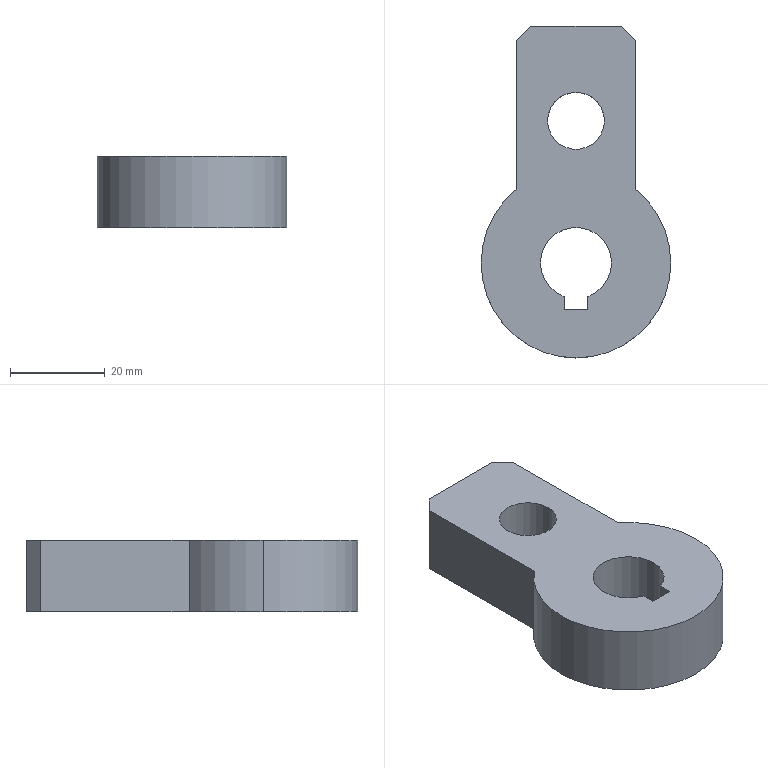Part | STEP file | 1 solid | 18 faces | box 40 x 70 x 15 mm | volume 25956 mm3 | plane 10 | cylinder 8 | commonest cylinder face diameters 15 x3 40 x3 12 x2
STEP:
#1=CARTESIAN_POINT('',(0.,0.,0.));
#2=DIRECTION('',(0.,0.,1.));
#3=DIRECTION('',(1.,0.,0.));
#4=AXIS2_PLACEMENT_3D('',#1,#2,#3);
#5=CARTESIAN_POINT('',(-6.,30.,7.5));
#6=VERTEX_POINT('',#5);
#7=CARTESIAN_POINT('',(-6.,30.,-7.5));
#8=VERTEX_POINT('',#7);
#9=CARTESIAN_POINT('',(-6.,30.,-7.5));
#10=DIRECTION('',(0.,0.,-1.));
#11=VECTOR('',#10,1.);
#12=LINE('',#9,#11);
#13=CARTESIAN_POINT('',(0.,30.,-7.5));
#14=DIRECTION('',(0.,0.,-1.));
#15=DIRECTION('',(-1.,0.,0.));
#16=AXIS2_PLACEMENT_3D('',#13,#14,#15);
#17=CYLINDRICAL_SURFACE('',#16,6.);
#18=CARTESIAN_POINT('',(6.283,0.));
#19=DIRECTION('',(0.,1.));
#20=VECTOR('',#19,1.);
#21=LINE('',#18,#20);
#22=(GEOMETRIC_REPRESENTATION_CONTEXT(2)PARAMETRIC_REPRESENTATION_CONTEXT()REPRESENTATION_CONTEXT('',''));
#23=DEFINITIONAL_REPRESENTATION('',(#21),#22);
#24=PCURVE('',#17,#23);
#25=CARTESIAN_POINT('',(0.,30.,-7.5));
#26=DIRECTION('',(0.,0.,-1.));
#27=DIRECTION('',(-1.,0.,0.));
#28=AXIS2_PLACEMENT_3D('',#25,#26,#27);
#29=CYLINDRICAL_SURFACE('',#28,6.);
#30=CARTESIAN_POINT('',(0.,0.));
#31=DIRECTION('',(0.,1.));
#32=VECTOR('',#31,1.);
#33=LINE('',#30,#32);
#34=(GEOMETRIC_REPRESENTATION_CONTEXT(2)PARAMETRIC_REPRESENTATION_CONTEXT()REPRESENTATION_CONTEXT('',''));
#35=DEFINITIONAL_REPRESENTATION('',(#33),#34);
#36=PCURVE('',#29,#35);
#37=SURFACE_CURVE('',#12,(#24,#36),.PCURVE_S1.);
#38=EDGE_CURVE('',#6,#8,#37,.T.);
#39=ORIENTED_EDGE('',*,*,#38,.T.);
#40=CARTESIAN_POINT('',(6.,30.,-7.5));
#41=VERTEX_POINT('',#40);
#42=CARTESIAN_POINT('',(0.,30.,-7.5));
#43=DIRECTION('',(0.,0.,1.));
#44=DIRECTION('',(-1.,0.,0.));
#45=AXIS2_PLACEMENT_3D('',#42,#43,#44);
#46=CIRCLE('',#45,6.);
#47=CARTESIAN_POINT('',(6.283,0.));
#48=DIRECTION('',(-1.,0.));
#49=VECTOR('',#48,1.);
#50=LINE('',#47,#49);
#51=(GEOMETRIC_REPRESENTATION_CONTEXT(2)PARAMETRIC_REPRESENTATION_CONTEXT()REPRESENTATION_CONTEXT('',''));
#52=DEFINITIONAL_REPRESENTATION('',(#50),#51);
#53=PCURVE('',#17,#52);
#54=CARTESIAN_POINT('',(0.,0.,-7.5));
#55=DIRECTION('',(0.,0.,1.));
#56=DIRECTION('',(1.,0.,0.));
#57=AXIS2_PLACEMENT_3D('',#54,#55,#56);
#58=PLANE('',#57);
#59=CARTESIAN_POINT('',(0.,30.));
#60=DIRECTION('',(-1.,0.));
#61=AXIS2_PLACEMENT_2D('',#59,#60);
#62=CIRCLE('',#61,6.);
#63=(GEOMETRIC_REPRESENTATION_CONTEXT(2)PARAMETRIC_REPRESENTATION_CONTEXT()REPRESENTATION_CONTEXT('',''));
#64=DEFINITIONAL_REPRESENTATION('',(#62),#63);
#65=PCURVE('',#58,#64);
#66=SURFACE_CURVE('',#46,(#53,#65),.PCURVE_S1.);
#67=EDGE_CURVE('',#8,#41,#66,.T.);
#68=ORIENTED_EDGE('',*,*,#67,.T.);
#69=CARTESIAN_POINT('',(6.,30.,7.5));
#70=VERTEX_POINT('',#69);
#71=CARTESIAN_POINT('',(6.,30.,-7.5));
#72=DIRECTION('',(0.,0.,-1.));
#73=VECTOR('',#72,1.);
#74=LINE('',#71,#73);
#75=CARTESIAN_POINT('',(3.142,0.));
#76=DIRECTION('',(0.,1.));
#77=VECTOR('',#76,1.);
#78=LINE('',#75,#77);
#79=(GEOMETRIC_REPRESENTATION_CONTEXT(2)PARAMETRIC_REPRESENTATION_CONTEXT()REPRESENTATION_CONTEXT('',''));
#80=DEFINITIONAL_REPRESENTATION('',(#78),#79);
#81=PCURVE('',#17,#80);
#82=CARTESIAN_POINT('',(3.142,0.));
#83=DIRECTION('',(0.,1.));
#84=VECTOR('',#83,1.);
#85=LINE('',#82,#84);
#86=(GEOMETRIC_REPRESENTATION_CONTEXT(2)PARAMETRIC_REPRESENTATION_CONTEXT()REPRESENTATION_CONTEXT('',''));
#87=DEFINITIONAL_REPRESENTATION('',(#85),#86);
#88=PCURVE('',#29,#87);
#89=SURFACE_CURVE('',#74,(#81,#88),.PCURVE_S1.);
#90=EDGE_CURVE('',#70,#41,#89,.T.);
#91=ORIENTED_EDGE('',*,*,#90,.F.);
#92=CARTESIAN_POINT('',(0.,30.,7.5));
#93=DIRECTION('',(0.,0.,-1.));
#94=DIRECTION('',(-1.,0.,0.));
#95=AXIS2_PLACEMENT_3D('',#92,#93,#94);
#96=CIRCLE('',#95,6.);
#97=CARTESIAN_POINT('',(0.,-15.));
#98=DIRECTION('',(1.,0.));
#99=VECTOR('',#98,1.);
#100=LINE('',#97,#99);
#101=(GEOMETRIC_REPRESENTATION_CONTEXT(2)PARAMETRIC_REPRESENTATION_CONTEXT()REPRESENTATION_CONTEXT('',''));
#102=DEFINITIONAL_REPRESENTATION('',(#100),#101);
#103=PCURVE('',#17,#102);
#104=CARTESIAN_POINT('',(0.,0.,7.5));
#105=DIRECTION('',(0.,0.,1.));
#106=DIRECTION('',(1.,0.,0.));
#107=AXIS2_PLACEMENT_3D('',#104,#105,#106);
#108=PLANE('',#107);
#109=CARTESIAN_POINT('',(-6.,30.));
#110=CARTESIAN_POINT('',(-6.,40.392));
#111=CARTESIAN_POINT('',(3.,35.196));
#112=CARTESIAN_POINT('',(12.,30.));
#113=CARTESIAN_POINT('',(3.,24.804));
#114=CARTESIAN_POINT('',(-6.,19.608));
#115=CARTESIAN_POINT('',(-6.,30.));
#116=(BOUNDED_CURVE()B_SPLINE_CURVE(2,(#109,#110,#111,#112,#113,#114,#115),.UNSPECIFIED.,.T.,.F.)B_SPLINE_CURVE_WITH_KNOTS((1,2,2,2,2,1),(-2.094,0.,2.094,4.189,6.283,8.378),.UNSPECIFIED.)CURVE()GEOMETRIC_REPRESENTATION_ITEM()RATIONAL_B_SPLINE_CURVE((1.,0.5,1.,0.5,1.,0.5,1.))REPRESENTATION_ITEM(''));
#117=(GEOMETRIC_REPRESENTATION_CONTEXT(2)PARAMETRIC_REPRESENTATION_CONTEXT()REPRESENTATION_CONTEXT('',''));
#118=DEFINITIONAL_REPRESENTATION('',(#116),#117);
#119=PCURVE('',#108,#118);
#120=SURFACE_CURVE('',#96,(#103,#119),.PCURVE_S1.);
#121=EDGE_CURVE('',#70,#6,#120,.T.);
#122=ORIENTED_EDGE('',*,*,#121,.T.);
#123=EDGE_LOOP('',(#39,#68,#91,#122));
#124=FACE_BOUND('',#123,.F.);
#125=ADVANCED_FACE('',(#124),#17,.F.);
#126=CARTESIAN_POINT('',(-2.5,-7.071,-7.5));
#127=VERTEX_POINT('',#126);
#128=CARTESIAN_POINT('',(-2.5,-7.071,7.5));
#129=VERTEX_POINT('',#128);
#130=CARTESIAN_POINT('',(-2.5,-7.071,7.5));
#131=DIRECTION('',(0.,0.,1.));
#132=VECTOR('',#131,1.);
#133=LINE('',#130,#132);
#134=CARTESIAN_POINT('',(0.,0.,7.5));
#135=DIRECTION('',(0.,0.,1.));
#136=DIRECTION('',(1.,0.,0.));
#137=AXIS2_PLACEMENT_3D('',#134,#135,#136);
#138=CYLINDRICAL_SURFACE('',#137,7.5);
#139=CARTESIAN_POINT('',(4.373,0.));
#140=DIRECTION('',(0.,1.));
#141=VECTOR('',#140,1.);
#142=LINE('',#139,#141);
#143=(GEOMETRIC_REPRESENTATION_CONTEXT(2)PARAMETRIC_REPRESENTATION_CONTEXT()REPRESENTATION_CONTEXT('',''));
#144=DEFINITIONAL_REPRESENTATION('',(#142),#143);
#145=PCURVE('',#138,#144);
#146=CARTESIAN_POINT('',(-2.5,-9.8,-7.5));
#147=DIRECTION('',(-1.,0.,0.));
#148=DIRECTION('',(0.,0.,1.));
#149=AXIS2_PLACEMENT_3D('',#146,#147,#148);
#150=PLANE('',#149);
#151=CARTESIAN_POINT('',(15.,2.729));
#152=DIRECTION('',(1.,0.));
#153=VECTOR('',#152,1.);
#154=LINE('',#151,#153);
#155=(GEOMETRIC_REPRESENTATION_CONTEXT(2)PARAMETRIC_REPRESENTATION_CONTEXT()REPRESENTATION_CONTEXT('',''));
#156=DEFINITIONAL_REPRESENTATION('',(#154),#155);
#157=PCURVE('',#150,#156);
#158=SURFACE_CURVE('',#133,(#145,#157),.PCURVE_S1.);
#159=EDGE_CURVE('',#127,#129,#158,.T.);
#160=ORIENTED_EDGE('',*,*,#159,.T.);
#161=CARTESIAN_POINT('',(-7.5,0.,7.5));
#162=VERTEX_POINT('',#161);
#163=CARTESIAN_POINT('',(0.,0.,7.5));
#164=DIRECTION('',(0.,0.,-1.));
#165=DIRECTION('',(1.,0.,0.));
#166=AXIS2_PLACEMENT_3D('',#163,#164,#165);
#167=CIRCLE('',#166,7.5);
#168=CARTESIAN_POINT('',(6.283,0.));
#169=DIRECTION('',(-1.,0.));
#170=VECTOR('',#169,1.);
#171=LINE('',#168,#170);
#172=(GEOMETRIC_REPRESENTATION_CONTEXT(2)PARAMETRIC_REPRESENTATION_CONTEXT()REPRESENTATION_CONTEXT('',''));
#173=DEFINITIONAL_REPRESENTATION('',(#171),#172);
#174=PCURVE('',#138,#173);
#175=CARTESIAN_POINT('',(7.5,0.));
#176=CARTESIAN_POINT('',(7.5,-12.99));
#177=CARTESIAN_POINT('',(-3.75,-6.495));
#178=CARTESIAN_POINT('',(-15.,0.));
#179=CARTESIAN_POINT('',(-3.75,6.495));
#180=CARTESIAN_POINT('',(7.5,12.99));
#181=CARTESIAN_POINT('',(7.5,0.));
#182=(BOUNDED_CURVE()B_SPLINE_CURVE(2,(#175,#176,#177,#178,#179,#180,#181),.UNSPECIFIED.,.T.,.F.)B_SPLINE_CURVE_WITH_KNOTS((1,2,2,2,2,1),(-2.094,0.,2.094,4.189,6.283,8.378),.UNSPECIFIED.)CURVE()GEOMETRIC_REPRESENTATION_ITEM()RATIONAL_B_SPLINE_CURVE((1.,0.5,1.,0.5,1.,0.5,1.))REPRESENTATION_ITEM(''));
#183=(GEOMETRIC_REPRESENTATION_CONTEXT(2)PARAMETRIC_REPRESENTATION_CONTEXT()REPRESENTATION_CONTEXT('',''));
#184=DEFINITIONAL_REPRESENTATION('',(#182),#183);
#185=PCURVE('',#108,#184);
#186=SURFACE_CURVE('',#167,(#174,#185),.PCURVE_S1.);
#187=EDGE_CURVE('',#129,#162,#186,.T.);
#188=ORIENTED_EDGE('',*,*,#187,.T.);
#189=CARTESIAN_POINT('',(-7.5,0.,-7.5));
#190=VERTEX_POINT('',#189);
#191=CARTESIAN_POINT('',(-7.5,0.,7.5));
#192=DIRECTION('',(0.,0.,1.));
#193=VECTOR('',#192,1.);
#194=LINE('',#191,#193);
#195=CARTESIAN_POINT('',(3.142,0.));
#196=DIRECTION('',(0.,1.));
#197=VECTOR('',#196,1.);
#198=LINE('',#195,#197);
#199=(GEOMETRIC_REPRESENTATION_CONTEXT(2)PARAMETRIC_REPRESENTATION_CONTEXT()REPRESENTATION_CONTEXT('',''));
#200=DEFINITIONAL_REPRESENTATION('',(#198),#199);
#201=PCURVE('',#138,#200);
#202=CARTESIAN_POINT('',(0.,0.,7.5));
#203=DIRECTION('',(0.,0.,1.));
#204=DIRECTION('',(1.,0.,0.));
#205=AXIS2_PLACEMENT_3D('',#202,#203,#204);
#206=CYLINDRICAL_SURFACE('',#205,7.5);
#207=CARTESIAN_POINT('',(3.142,0.));
#208=DIRECTION('',(0.,1.));
#209=VECTOR('',#208,1.);
#210=LINE('',#207,#209);
#211=(GEOMETRIC_REPRESENTATION_CONTEXT(2)PARAMETRIC_REPRESENTATION_CONTEXT()REPRESENTATION_CONTEXT('',''));
#212=DEFINITIONAL_REPRESENTATION('',(#210),#211);
#213=PCURVE('',#206,#212);
#214=SURFACE_CURVE('',#194,(#201,#213),.PCURVE_S1.);
#215=EDGE_CURVE('',#190,#162,#214,.T.);
#216=ORIENTED_EDGE('',*,*,#215,.F.);
#217=CARTESIAN_POINT('',(0.,0.,-7.5));
#218=DIRECTION('',(0.,0.,1.));
#219=DIRECTION('',(1.,0.,0.));
#220=AXIS2_PLACEMENT_3D('',#217,#218,#219);
#221=CIRCLE('',#220,7.5);
#222=CARTESIAN_POINT('',(0.,-15.));
#223=DIRECTION('',(1.,0.));
#224=VECTOR('',#223,1.);
#225=LINE('',#222,#224);
#226=(GEOMETRIC_REPRESENTATION_CONTEXT(2)PARAMETRIC_REPRESENTATION_CONTEXT()REPRESENTATION_CONTEXT('',''));
#227=DEFINITIONAL_REPRESENTATION('',(#225),#226);
#228=PCURVE('',#138,#227);
#229=CARTESIAN_POINT('',(0.,0.));
#230=DIRECTION('',(1.,0.));
#231=AXIS2_PLACEMENT_2D('',#229,#230);
#232=CIRCLE('',#231,7.5);
#233=(GEOMETRIC_REPRESENTATION_CONTEXT(2)PARAMETRIC_REPRESENTATION_CONTEXT()REPRESENTATION_CONTEXT('',''));
#234=DEFINITIONAL_REPRESENTATION('',(#232),#233);
#235=PCURVE('',#58,#234);
#236=SURFACE_CURVE('',#221,(#228,#235),.PCURVE_S1.);
#237=EDGE_CURVE('',#190,#127,#236,.T.);
#238=ORIENTED_EDGE('',*,*,#237,.T.);
#239=EDGE_LOOP('',(#160,#188,#216,#238));
#240=FACE_BOUND('',#239,.F.);
#241=ADVANCED_FACE('',(#240),#138,.F.);
#242=CARTESIAN_POINT('',(7.5,0.,7.5));
#243=VERTEX_POINT('',#242);
#244=CARTESIAN_POINT('',(0.,0.,7.5));
#245=DIRECTION('',(0.,0.,-1.));
#246=DIRECTION('',(1.,0.,0.));
#247=AXIS2_PLACEMENT_3D('',#244,#245,#246);
#248=CIRCLE('',#247,7.5);
#249=CARTESIAN_POINT('',(6.283,0.));
#250=DIRECTION('',(-1.,0.));
#251=VECTOR('',#250,1.);
#252=LINE('',#249,#251);
#253=(GEOMETRIC_REPRESENTATION_CONTEXT(2)PARAMETRIC_REPRESENTATION_CONTEXT()REPRESENTATION_CONTEXT('',''));
#254=DEFINITIONAL_REPRESENTATION('',(#252),#253);
#255=PCURVE('',#206,#254);
#256=CARTESIAN_POINT('',(7.5,0.));
#257=CARTESIAN_POINT('',(7.5,-12.99));
#258=CARTESIAN_POINT('',(-3.75,-6.495));
#259=CARTESIAN_POINT('',(-15.,0.));
#260=CARTESIAN_POINT('',(-3.75,6.495));
#261=CARTESIAN_POINT('',(7.5,12.99));
#262=CARTESIAN_POINT('',(7.5,0.));
#263=(BOUNDED_CURVE()B_SPLINE_CURVE(2,(#256,#257,#258,#259,#260,#261,#262),.UNSPECIFIED.,.T.,.F.)B_SPLINE_CURVE_WITH_KNOTS((1,2,2,2,2,1),(-2.094,0.,2.094,4.189,6.283,8.378),.UNSPECIFIED.)CURVE()GEOMETRIC_REPRESENTATION_ITEM()RATIONAL_B_SPLINE_CURVE((1.,0.5,1.,0.5,1.,0.5,1.))REPRESENTATION_ITEM(''));
#264=(GEOMETRIC_REPRESENTATION_CONTEXT(2)PARAMETRIC_REPRESENTATION_CONTEXT()REPRESENTATION_CONTEXT('',''));
#265=DEFINITIONAL_REPRESENTATION('',(#263),#264);
#266=PCURVE('',#108,#265);
#267=SURFACE_CURVE('',#248,(#255,#266),.PCURVE_S1.);
#268=EDGE_CURVE('',#162,#243,#267,.T.);
#269=ORIENTED_EDGE('',*,*,#268,.T.);
#270=CARTESIAN_POINT('',(7.5,0.,-7.5));
#271=VERTEX_POINT('',#270);
#272=CARTESIAN_POINT('',(7.5,0.,7.5));
#273=DIRECTION('',(0.,0.,1.));
#274=VECTOR('',#273,1.);
#275=LINE('',#272,#274);
#276=CARTESIAN_POINT('',(0.,0.));
#277=DIRECTION('',(0.,1.));
#278=VECTOR('',#277,1.);
#279=LINE('',#276,#278);
#280=(GEOMETRIC_REPRESENTATION_CONTEXT(2)PARAMETRIC_REPRESENTATION_CONTEXT()REPRESENTATION_CONTEXT('',''));
#281=DEFINITIONAL_REPRESENTATION('',(#279),#280);
#282=PCURVE('',#206,#281);
#283=CARTESIAN_POINT('',(0.,0.,7.5));
#284=DIRECTION('',(0.,0.,1.));
#285=DIRECTION('',(1.,0.,0.));
#286=AXIS2_PLACEMENT_3D('',#283,#284,#285);
#287=CYLINDRICAL_SURFACE('',#286,7.5);
#288=CARTESIAN_POINT('',(6.283,0.));
#289=DIRECTION('',(0.,1.));
#290=VECTOR('',#289,1.);
#291=LINE('',#288,#290);
#292=(GEOMETRIC_REPRESENTATION_CONTEXT(2)PARAMETRIC_REPRESENTATION_CONTEXT()REPRESENTATION_CONTEXT('',''));
#293=DEFINITIONAL_REPRESENTATION('',(#291),#292);
#294=PCURVE('',#287,#293);
#295=SURFACE_CURVE('',#275,(#282,#294),.PCURVE_S1.);
#296=EDGE_CURVE('',#271,#243,#295,.T.);
#297=ORIENTED_EDGE('',*,*,#296,.F.);
#298=CARTESIAN_POINT('',(0.,0.,-7.5));
#299=DIRECTION('',(0.,0.,1.));
#300=DIRECTION('',(1.,0.,0.));
#301=AXIS2_PLACEMENT_3D('',#298,#299,#300);
#302=CIRCLE('',#301,7.5);
#303=CARTESIAN_POINT('',(0.,-15.));
#304=DIRECTION('',(1.,0.));
#305=VECTOR('',#304,1.);
#306=LINE('',#303,#305);
#307=(GEOMETRIC_REPRESENTATION_CONTEXT(2)PARAMETRIC_REPRESENTATION_CONTEXT()REPRESENTATION_CONTEXT('',''));
#308=DEFINITIONAL_REPRESENTATION('',(#306),#307);
#309=PCURVE('',#206,#308);
#310=CARTESIAN_POINT('',(0.,0.));
#311=DIRECTION('',(1.,0.));
#312=AXIS2_PLACEMENT_2D('',#310,#311);
#313=CIRCLE('',#312,7.5);
#314=(GEOMETRIC_REPRESENTATION_CONTEXT(2)PARAMETRIC_REPRESENTATION_CONTEXT()REPRESENTATION_CONTEXT('',''));
#315=DEFINITIONAL_REPRESENTATION('',(#313),#314);
#316=PCURVE('',#58,#315);
#317=SURFACE_CURVE('',#302,(#309,#316),.PCURVE_S1.);
#318=EDGE_CURVE('',#271,#190,#317,.T.);
#319=ORIENTED_EDGE('',*,*,#318,.T.);
#320=ORIENTED_EDGE('',*,*,#215,.T.);
#321=EDGE_LOOP('',(#269,#297,#319,#320));
#322=FACE_BOUND('',#321,.F.);
#323=ADVANCED_FACE('',(#322),#206,.F.);
#324=CARTESIAN_POINT('',(-12.5,15.612,-7.5));
#325=VERTEX_POINT('',#324);
#326=CARTESIAN_POINT('',(-20.,0.,-7.5));
#327=VERTEX_POINT('',#326);
#328=CARTESIAN_POINT('',(0.,0.,-7.5));
#329=DIRECTION('',(0.,0.,1.));
#330=DIRECTION('',(1.,0.,0.));
#331=AXIS2_PLACEMENT_3D('',#328,#329,#330);
#332=CIRCLE('',#331,20.);
#333=CARTESIAN_POINT('',(0.,0.,7.5));
#334=DIRECTION('',(0.,0.,1.));
#335=DIRECTION('',(1.,0.,0.));
#336=AXIS2_PLACEMENT_3D('',#333,#334,#335);
#337=CYLINDRICAL_SURFACE('',#336,20.);
#338=CARTESIAN_POINT('',(0.,-15.));
#339=DIRECTION('',(1.,0.));
#340=VECTOR('',#339,1.);
#341=LINE('',#338,#340);
#342=(GEOMETRIC_REPRESENTATION_CONTEXT(2)PARAMETRIC_REPRESENTATION_CONTEXT()REPRESENTATION_CONTEXT('',''));
#343=DEFINITIONAL_REPRESENTATION('',(#341),#342);
#344=PCURVE('',#337,#343);
#345=CARTESIAN_POINT('',(0.,0.));
#346=DIRECTION('',(1.,0.));
#347=AXIS2_PLACEMENT_2D('',#345,#346);
#348=CIRCLE('',#347,20.);
#349=(GEOMETRIC_REPRESENTATION_CONTEXT(2)PARAMETRIC_REPRESENTATION_CONTEXT()REPRESENTATION_CONTEXT('',''));
#350=DEFINITIONAL_REPRESENTATION('',(#348),#349);
#351=PCURVE('',#58,#350);
#352=SURFACE_CURVE('',#332,(#344,#351),.PCURVE_S1.);
#353=EDGE_CURVE('',#325,#327,#352,.T.);
#354=ORIENTED_EDGE('',*,*,#353,.T.);
#355=CARTESIAN_POINT('',(-20.,0.,7.5));
#356=VERTEX_POINT('',#355);
#357=CARTESIAN_POINT('',(-20.,0.,7.5));
#358=DIRECTION('',(0.,0.,1.));
#359=VECTOR('',#358,1.);
#360=LINE('',#357,#359);
#361=CARTESIAN_POINT('',(3.142,0.));
#362=DIRECTION('',(0.,1.));
#363=VECTOR('',#362,1.);
#364=LINE('',#361,#363);
#365=(GEOMETRIC_REPRESENTATION_CONTEXT(2)PARAMETRIC_REPRESENTATION_CONTEXT()REPRESENTATION_CONTEXT('',''));
#366=DEFINITIONAL_REPRESENTATION('',(#364),#365);
#367=PCURVE('',#337,#366);
#368=CARTESIAN_POINT('',(0.,0.,7.5));
#369=DIRECTION('',(0.,0.,1.));
#370=DIRECTION('',(1.,0.,0.));
#371=AXIS2_PLACEMENT_3D('',#368,#369,#370);
#372=CYLINDRICAL_SURFACE('',#371,20.);
#373=CARTESIAN_POINT('',(3.142,0.));
#374=DIRECTION('',(0.,1.));
#375=VECTOR('',#374,1.);
#376=LINE('',#373,#375);
#377=(GEOMETRIC_REPRESENTATION_CONTEXT(2)PARAMETRIC_REPRESENTATION_CONTEXT()REPRESENTATION_CONTEXT('',''));
#378=DEFINITIONAL_REPRESENTATION('',(#376),#377);
#379=PCURVE('',#372,#378);
#380=SURFACE_CURVE('',#360,(#367,#379),.PCURVE_S1.);
#381=EDGE_CURVE('',#327,#356,#380,.T.);
#382=ORIENTED_EDGE('',*,*,#381,.T.);
#383=CARTESIAN_POINT('',(-12.5,15.612,7.5));
#384=VERTEX_POINT('',#383);
#385=CARTESIAN_POINT('',(0.,0.,7.5));
#386=DIRECTION('',(0.,0.,1.));
#387=DIRECTION('',(1.,0.,0.));
#388=AXIS2_PLACEMENT_3D('',#385,#386,#387);
#389=CIRCLE('',#388,20.);
#390=CARTESIAN_POINT('',(0.,0.));
#391=DIRECTION('',(1.,0.));
#392=VECTOR('',#391,1.);
#393=LINE('',#390,#392);
#394=(GEOMETRIC_REPRESENTATION_CONTEXT(2)PARAMETRIC_REPRESENTATION_CONTEXT()REPRESENTATION_CONTEXT('',''));
#395=DEFINITIONAL_REPRESENTATION('',(#393),#394);
#396=PCURVE('',#337,#395);
#397=CARTESIAN_POINT('',(0.,0.));
#398=DIRECTION('',(1.,0.));
#399=AXIS2_PLACEMENT_2D('',#397,#398);
#400=CIRCLE('',#399,20.);
#401=(GEOMETRIC_REPRESENTATION_CONTEXT(2)PARAMETRIC_REPRESENTATION_CONTEXT()REPRESENTATION_CONTEXT('',''));
#402=DEFINITIONAL_REPRESENTATION('',(#400),#401);
#403=PCURVE('',#108,#402);
#404=SURFACE_CURVE('',#389,(#396,#403),.PCURVE_S1.);
#405=EDGE_CURVE('',#384,#356,#404,.T.);
#406=ORIENTED_EDGE('',*,*,#405,.F.);
#407=CARTESIAN_POINT('',(-12.5,15.612,7.5));
#408=DIRECTION('',(0.,0.,-1.));
#409=VECTOR('',#408,1.);
#410=LINE('',#407,#409);
#411=CARTESIAN_POINT('',(2.246,0.));
#412=DIRECTION('',(0.,-1.));
#413=VECTOR('',#412,1.);
#414=LINE('',#411,#413);
#415=(GEOMETRIC_REPRESENTATION_CONTEXT(2)PARAMETRIC_REPRESENTATION_CONTEXT()REPRESENTATION_CONTEXT('',''));
#416=DEFINITIONAL_REPRESENTATION('',(#414),#415);
#417=PCURVE('',#337,#416);
#418=CARTESIAN_POINT('',(-12.5,50.,7.5));
#419=DIRECTION('',(1.,0.,0.));
#420=DIRECTION('',(0.,1.,0.));
#421=AXIS2_PLACEMENT_3D('',#418,#419,#420);
#422=PLANE('',#421);
#423=CARTESIAN_POINT('',(-34.388,0.));
#424=DIRECTION('',(0.,-1.));
#425=VECTOR('',#424,1.);
#426=LINE('',#423,#425);
#427=(GEOMETRIC_REPRESENTATION_CONTEXT(2)PARAMETRIC_REPRESENTATION_CONTEXT()REPRESENTATION_CONTEXT('',''));
#428=DEFINITIONAL_REPRESENTATION('',(#426),#427);
#429=PCURVE('',#422,#428);
#430=SURFACE_CURVE('',#410,(#417,#429),.PCURVE_S1.);
#431=EDGE_CURVE('',#384,#325,#430,.T.);
#432=ORIENTED_EDGE('',*,*,#431,.T.);
#433=EDGE_LOOP('',(#354,#382,#406,#432));
#434=FACE_BOUND('',#433,.T.);
#435=ADVANCED_FACE('',(#434),#337,.T.);
#436=ORIENTED_EDGE('',*,*,#381,.F.);
#437=CARTESIAN_POINT('',(20.,0.,-7.5));
#438=VERTEX_POINT('',#437);
#439=CARTESIAN_POINT('',(0.,0.,-7.5));
#440=DIRECTION('',(0.,0.,1.));
#441=DIRECTION('',(1.,0.,0.));
#442=AXIS2_PLACEMENT_3D('',#439,#440,#441);
#443=CIRCLE('',#442,20.);
#444=CARTESIAN_POINT('',(0.,-15.));
#445=DIRECTION('',(1.,0.));
#446=VECTOR('',#445,1.);
#447=LINE('',#444,#446);
#448=(GEOMETRIC_REPRESENTATION_CONTEXT(2)PARAMETRIC_REPRESENTATION_CONTEXT()REPRESENTATION_CONTEXT('',''));
#449=DEFINITIONAL_REPRESENTATION('',(#447),#448);
#450=PCURVE('',#372,#449);
#451=CARTESIAN_POINT('',(0.,0.));
#452=DIRECTION('',(1.,0.));
#453=AXIS2_PLACEMENT_2D('',#451,#452);
#454=CIRCLE('',#453,20.);
#455=(GEOMETRIC_REPRESENTATION_CONTEXT(2)PARAMETRIC_REPRESENTATION_CONTEXT()REPRESENTATION_CONTEXT('',''));
#456=DEFINITIONAL_REPRESENTATION('',(#454),#455);
#457=PCURVE('',#58,#456);
#458=SURFACE_CURVE('',#443,(#450,#457),.PCURVE_S1.);
#459=EDGE_CURVE('',#327,#438,#458,.T.);
#460=ORIENTED_EDGE('',*,*,#459,.T.);
#461=CARTESIAN_POINT('',(20.,0.,7.5));
#462=VERTEX_POINT('',#461);
#463=CARTESIAN_POINT('',(20.,0.,7.5));
#464=DIRECTION('',(0.,0.,1.));
#465=VECTOR('',#464,1.);
#466=LINE('',#463,#465);
#467=CARTESIAN_POINT('',(6.283,0.));
#468=DIRECTION('',(0.,1.));
#469=VECTOR('',#468,1.);
#470=LINE('',#467,#469);
#471=(GEOMETRIC_REPRESENTATION_CONTEXT(2)PARAMETRIC_REPRESENTATION_CONTEXT()REPRESENTATION_CONTEXT('',''));
#472=DEFINITIONAL_REPRESENTATION('',(#470),#471);
#473=PCURVE('',#372,#472);
#474=CARTESIAN_POINT('',(0.,0.,7.5));
#475=DIRECTION('',(0.,0.,1.));
#476=DIRECTION('',(1.,0.,0.));
#477=AXIS2_PLACEMENT_3D('',#474,#475,#476);
#478=CYLINDRICAL_SURFACE('',#477,20.);
#479=CARTESIAN_POINT('',(0.,0.));
#480=DIRECTION('',(0.,1.));
#481=VECTOR('',#480,1.);
#482=LINE('',#479,#481);
#483=(GEOMETRIC_REPRESENTATION_CONTEXT(2)PARAMETRIC_REPRESENTATION_CONTEXT()REPRESENTATION_CONTEXT('',''));
#484=DEFINITIONAL_REPRESENTATION('',(#482),#483);
#485=PCURVE('',#478,#484);
#486=SURFACE_CURVE('',#466,(#473,#485),.PCURVE_S1.);
#487=EDGE_CURVE('',#438,#462,#486,.T.);
#488=ORIENTED_EDGE('',*,*,#487,.T.);
#489=CARTESIAN_POINT('',(0.,0.,7.5));
#490=DIRECTION('',(0.,0.,1.));
#491=DIRECTION('',(1.,0.,0.));
#492=AXIS2_PLACEMENT_3D('',#489,#490,#491);
#493=CIRCLE('',#492,20.);
#494=CARTESIAN_POINT('',(0.,0.));
#495=DIRECTION('',(1.,0.));
#496=VECTOR('',#495,1.);
#497=LINE('',#494,#496);
#498=(GEOMETRIC_REPRESENTATION_CONTEXT(2)PARAMETRIC_REPRESENTATION_CONTEXT()REPRESENTATION_CONTEXT('',''));
#499=DEFINITIONAL_REPRESENTATION('',(#497),#498);
#500=PCURVE('',#372,#499);
#501=CARTESIAN_POINT('',(0.,0.));
#502=DIRECTION('',(1.,0.));
#503=AXIS2_PLACEMENT_2D('',#501,#502);
#504=CIRCLE('',#503,20.);
#505=(GEOMETRIC_REPRESENTATION_CONTEXT(2)PARAMETRIC_REPRESENTATION_CONTEXT()REPRESENTATION_CONTEXT('',''));
#506=DEFINITIONAL_REPRESENTATION('',(#504),#505);
#507=PCURVE('',#108,#506);
#508=SURFACE_CURVE('',#493,(#500,#507),.PCURVE_S1.);
#509=EDGE_CURVE('',#356,#462,#508,.T.);
#510=ORIENTED_EDGE('',*,*,#509,.F.);
#511=EDGE_LOOP('',(#436,#460,#488,#510));
#512=FACE_BOUND('',#511,.T.);
#513=ADVANCED_FACE('',(#512),#372,.T.);
#514=CARTESIAN_POINT('',(0.,30.,7.5));
#515=DIRECTION('',(0.,0.,-1.));
#516=DIRECTION('',(-1.,0.,0.));
#517=AXIS2_PLACEMENT_3D('',#514,#515,#516);
#518=CIRCLE('',#517,6.);
#519=CARTESIAN_POINT('',(-6.,30.));
#520=CARTESIAN_POINT('',(-6.,40.392));
#521=CARTESIAN_POINT('',(3.,35.196));
#522=CARTESIAN_POINT('',(12.,30.));
#523=CARTESIAN_POINT('',(3.,24.804));
#524=CARTESIAN_POINT('',(-6.,19.608));
#525=CARTESIAN_POINT('',(-6.,30.));
#526=(BOUNDED_CURVE()B_SPLINE_CURVE(2,(#519,#520,#521,#522,#523,#524,#525),.UNSPECIFIED.,.T.,.F.)B_SPLINE_CURVE_WITH_KNOTS((1,2,2,2,2,1),(-2.094,0.,2.094,4.189,6.283,8.378),.UNSPECIFIED.)CURVE()GEOMETRIC_REPRESENTATION_ITEM()RATIONAL_B_SPLINE_CURVE((1.,0.5,1.,0.5,1.,0.5,1.))REPRESENTATION_ITEM(''));
#527=(GEOMETRIC_REPRESENTATION_CONTEXT(2)PARAMETRIC_REPRESENTATION_CONTEXT()REPRESENTATION_CONTEXT('',''));
#528=DEFINITIONAL_REPRESENTATION('',(#526),#527);
#529=PCURVE('',#108,#528);
#530=CARTESIAN_POINT('',(0.,-15.));
#531=DIRECTION('',(1.,0.));
#532=VECTOR('',#531,1.);
#533=LINE('',#530,#532);
#534=(GEOMETRIC_REPRESENTATION_CONTEXT(2)PARAMETRIC_REPRESENTATION_CONTEXT()REPRESENTATION_CONTEXT('',''));
#535=DEFINITIONAL_REPRESENTATION('',(#533),#534);
#536=PCURVE('',#29,#535);
#537=SURFACE_CURVE('',#518,(#529,#536),.PCURVE_S1.);
#538=EDGE_CURVE('',#6,#70,#537,.T.);
#539=ORIENTED_EDGE('',*,*,#538,.T.);
#540=ORIENTED_EDGE('',*,*,#121,.T.);
#541=EDGE_LOOP('',(#539,#540));
#542=FACE_BOUND('',#541,.T.);
#543=ORIENTED_EDGE('',*,*,#187,.T.);
#544=ORIENTED_EDGE('',*,*,#268,.T.);
#545=CARTESIAN_POINT('',(2.5,-7.071,7.5));
#546=VERTEX_POINT('',#545);
#547=CARTESIAN_POINT('',(0.,0.,7.5));
#548=DIRECTION('',(0.,0.,-1.));
#549=DIRECTION('',(1.,0.,0.));
#550=AXIS2_PLACEMENT_3D('',#547,#548,#549);
#551=CIRCLE('',#550,7.5);
#552=CARTESIAN_POINT('',(7.5,0.));
#553=CARTESIAN_POINT('',(7.5,-12.99));
#554=CARTESIAN_POINT('',(-3.75,-6.495));
#555=CARTESIAN_POINT('',(-15.,0.));
#556=CARTESIAN_POINT('',(-3.75,6.495));
#557=CARTESIAN_POINT('',(7.5,12.99));
#558=CARTESIAN_POINT('',(7.5,0.));
#559=(BOUNDED_CURVE()B_SPLINE_CURVE(2,(#552,#553,#554,#555,#556,#557,#558),.UNSPECIFIED.,.T.,.F.)B_SPLINE_CURVE_WITH_KNOTS((1,2,2,2,2,1),(-2.094,0.,2.094,4.189,6.283,8.378),.UNSPECIFIED.)CURVE()GEOMETRIC_REPRESENTATION_ITEM()RATIONAL_B_SPLINE_CURVE((1.,0.5,1.,0.5,1.,0.5,1.))REPRESENTATION_ITEM(''));
#560=(GEOMETRIC_REPRESENTATION_CONTEXT(2)PARAMETRIC_REPRESENTATION_CONTEXT()REPRESENTATION_CONTEXT('',''));
#561=DEFINITIONAL_REPRESENTATION('',(#559),#560);
#562=PCURVE('',#108,#561);
#563=CARTESIAN_POINT('',(6.283,0.));
#564=DIRECTION('',(-1.,0.));
#565=VECTOR('',#564,1.);
#566=LINE('',#563,#565);
#567=(GEOMETRIC_REPRESENTATION_CONTEXT(2)PARAMETRIC_REPRESENTATION_CONTEXT()REPRESENTATION_CONTEXT('',''));
#568=DEFINITIONAL_REPRESENTATION('',(#566),#567);
#569=PCURVE('',#287,#568);
#570=SURFACE_CURVE('',#551,(#562,#569),.PCURVE_S1.);
#571=EDGE_CURVE('',#243,#546,#570,.T.);
#572=ORIENTED_EDGE('',*,*,#571,.T.);
#573=CARTESIAN_POINT('',(2.5,-9.8,7.5));
#574=VERTEX_POINT('',#573);
#575=CARTESIAN_POINT('',(2.5,0.,7.5));
#576=DIRECTION('',(0.,-1.,0.));
#577=VECTOR('',#576,1.);
#578=LINE('',#575,#577);
#579=CARTESIAN_POINT('',(2.5,0.));
#580=DIRECTION('',(0.,-1.));
#581=VECTOR('',#580,1.);
#582=LINE('',#579,#581);
#583=(GEOMETRIC_REPRESENTATION_CONTEXT(2)PARAMETRIC_REPRESENTATION_CONTEXT()REPRESENTATION_CONTEXT('',''));
#584=DEFINITIONAL_REPRESENTATION('',(#582),#583);
#585=PCURVE('',#108,#584);
#586=CARTESIAN_POINT('',(2.5,-9.8,-7.5));
#587=DIRECTION('',(1.,0.,0.));
#588=DIRECTION('',(0.,0.,-1.));
#589=AXIS2_PLACEMENT_3D('',#586,#587,#588);
#590=PLANE('',#589);
#591=CARTESIAN_POINT('',(-15.,9.8));
#592=DIRECTION('',(0.,-1.));
#593=VECTOR('',#592,1.);
#594=LINE('',#591,#593);
#595=(GEOMETRIC_REPRESENTATION_CONTEXT(2)PARAMETRIC_REPRESENTATION_CONTEXT()REPRESENTATION_CONTEXT('',''));
#596=DEFINITIONAL_REPRESENTATION('',(#594),#595);
#597=PCURVE('',#590,#596);
#598=SURFACE_CURVE('',#578,(#585,#597),.PCURVE_S1.);
#599=EDGE_CURVE('',#546,#574,#598,.T.);
#600=ORIENTED_EDGE('',*,*,#599,.T.);
#601=CARTESIAN_POINT('',(-2.5,-9.8,7.5));
#602=VERTEX_POINT('',#601);
#603=CARTESIAN_POINT('',(0.,-9.8,7.5));
#604=DIRECTION('',(-1.,0.,0.));
#605=VECTOR('',#604,1.);
#606=LINE('',#603,#605);
#607=CARTESIAN_POINT('',(0.,-9.8));
#608=DIRECTION('',(-1.,0.));
#609=VECTOR('',#608,1.);
#610=LINE('',#607,#609);
#611=(GEOMETRIC_REPRESENTATION_CONTEXT(2)PARAMETRIC_REPRESENTATION_CONTEXT()REPRESENTATION_CONTEXT('',''));
#612=DEFINITIONAL_REPRESENTATION('',(#610),#611);
#613=PCURVE('',#108,#612);
#614=CARTESIAN_POINT('',(-2.5,-9.8,-7.5));
#615=DIRECTION('',(0.,-1.,0.));
#616=DIRECTION('',(0.,0.,-1.));
#617=AXIS2_PLACEMENT_3D('',#614,#615,#616);
#618=PLANE('',#617);
#619=CARTESIAN_POINT('',(-15.,2.5));
#620=DIRECTION('',(0.,-1.));
#621=VECTOR('',#620,1.);
#622=LINE('',#619,#621);
#623=(GEOMETRIC_REPRESENTATION_CONTEXT(2)PARAMETRIC_REPRESENTATION_CONTEXT()REPRESENTATION_CONTEXT('',''));
#624=DEFINITIONAL_REPRESENTATION('',(#622),#623);
#625=PCURVE('',#618,#624);
#626=SURFACE_CURVE('',#606,(#613,#625),.PCURVE_S1.);
#627=EDGE_CURVE('',#574,#602,#626,.T.);
#628=ORIENTED_EDGE('',*,*,#627,.T.);
#629=CARTESIAN_POINT('',(-2.5,0.,7.5));
#630=DIRECTION('',(0.,1.,0.));
#631=VECTOR('',#630,1.);
#632=LINE('',#629,#631);
#633=CARTESIAN_POINT('',(-2.5,0.));
#634=DIRECTION('',(0.,1.));
#635=VECTOR('',#634,1.);
#636=LINE('',#633,#635);
#637=(GEOMETRIC_REPRESENTATION_CONTEXT(2)PARAMETRIC_REPRESENTATION_CONTEXT()REPRESENTATION_CONTEXT('',''));
#638=DEFINITIONAL_REPRESENTATION('',(#636),#637);
#639=PCURVE('',#108,#638);
#640=CARTESIAN_POINT('',(15.,9.8));
#641=DIRECTION('',(0.,1.));
#642=VECTOR('',#641,1.);
#643=LINE('',#640,#642);
#644=(GEOMETRIC_REPRESENTATION_CONTEXT(2)PARAMETRIC_REPRESENTATION_CONTEXT()REPRESENTATION_CONTEXT('',''));
#645=DEFINITIONAL_REPRESENTATION('',(#643),#644);
#646=PCURVE('',#150,#645);
#647=SURFACE_CURVE('',#632,(#639,#646),.PCURVE_S1.);
#648=EDGE_CURVE('',#602,#129,#647,.T.);
#649=ORIENTED_EDGE('',*,*,#648,.T.);
#650=EDGE_LOOP('',(#543,#544,#572,#600,#628,#649));
#651=FACE_BOUND('',#650,.T.);
#652=ORIENTED_EDGE('',*,*,#405,.T.);
#653=ORIENTED_EDGE('',*,*,#509,.T.);
#654=CARTESIAN_POINT('',(12.5,15.612,7.5));
#655=VERTEX_POINT('',#654);
#656=CARTESIAN_POINT('',(0.,0.,7.5));
#657=DIRECTION('',(0.,0.,1.));
#658=DIRECTION('',(1.,0.,0.));
#659=AXIS2_PLACEMENT_3D('',#656,#657,#658);
#660=CIRCLE('',#659,20.);
#661=CARTESIAN_POINT('',(0.,0.));
#662=DIRECTION('',(1.,0.));
#663=AXIS2_PLACEMENT_2D('',#661,#662);
#664=CIRCLE('',#663,20.);
#665=(GEOMETRIC_REPRESENTATION_CONTEXT(2)PARAMETRIC_REPRESENTATION_CONTEXT()REPRESENTATION_CONTEXT('',''));
#666=DEFINITIONAL_REPRESENTATION('',(#664),#665);
#667=PCURVE('',#108,#666);
#668=CARTESIAN_POINT('',(0.,0.));
#669=DIRECTION('',(1.,0.));
#670=VECTOR('',#669,1.);
#671=LINE('',#668,#670);
#672=(GEOMETRIC_REPRESENTATION_CONTEXT(2)PARAMETRIC_REPRESENTATION_CONTEXT()REPRESENTATION_CONTEXT('',''));
#673=DEFINITIONAL_REPRESENTATION('',(#671),#672);
#674=PCURVE('',#478,#673);
#675=SURFACE_CURVE('',#660,(#667,#674),.PCURVE_S1.);
#676=EDGE_CURVE('',#462,#655,#675,.T.);
#677=ORIENTED_EDGE('',*,*,#676,.T.);
#678=CARTESIAN_POINT('',(12.5,47.,7.5));
#679=VERTEX_POINT('',#678);
#680=CARTESIAN_POINT('',(12.5,0.,7.5));
#681=DIRECTION('',(0.,1.,0.));
#682=VECTOR('',#681,1.);
#683=LINE('',#680,#682);
#684=CARTESIAN_POINT('',(12.5,0.));
#685=DIRECTION('',(0.,1.));
#686=VECTOR('',#685,1.);
#687=LINE('',#684,#686);
#688=(GEOMETRIC_REPRESENTATION_CONTEXT(2)PARAMETRIC_REPRESENTATION_CONTEXT()REPRESENTATION_CONTEXT('',''));
#689=DEFINITIONAL_REPRESENTATION('',(#687),#688);
#690=PCURVE('',#108,#689);
#691=CARTESIAN_POINT('',(12.5,50.,7.5));
#692=DIRECTION('',(-1.,0.,0.));
#693=DIRECTION('',(0.,-1.,0.));
#694=AXIS2_PLACEMENT_3D('',#691,#692,#693);
#695=PLANE('',#694);
#696=CARTESIAN_POINT('',(50.,0.));
#697=DIRECTION('',(-1.,0.));
#698=VECTOR('',#697,1.);
#699=LINE('',#696,#698);
#700=(GEOMETRIC_REPRESENTATION_CONTEXT(2)PARAMETRIC_REPRESENTATION_CONTEXT()REPRESENTATION_CONTEXT('',''));
#701=DEFINITIONAL_REPRESENTATION('',(#699),#700);
#702=PCURVE('',#695,#701);
#703=SURFACE_CURVE('',#683,(#690,#702),.PCURVE_S1.);
#704=EDGE_CURVE('',#655,#679,#703,.T.);
#705=ORIENTED_EDGE('',*,*,#704,.T.);
#706=CARTESIAN_POINT('',(9.5,50.,7.5));
#707=VERTEX_POINT('',#706);
#708=CARTESIAN_POINT('',(12.5,47.,7.5));
#709=DIRECTION('',(-0.7071,0.7071,0.));
#710=VECTOR('',#709,1.);
#711=LINE('',#708,#710);
#712=CARTESIAN_POINT('',(12.5,47.));
#713=DIRECTION('',(-0.7071,0.7071));
#714=VECTOR('',#713,1.);
#715=LINE('',#712,#714);
#716=(GEOMETRIC_REPRESENTATION_CONTEXT(2)PARAMETRIC_REPRESENTATION_CONTEXT()REPRESENTATION_CONTEXT('',''));
#717=DEFINITIONAL_REPRESENTATION('',(#715),#716);
#718=PCURVE('',#108,#717);
#719=CARTESIAN_POINT('',(9.5,50.,7.5));
#720=DIRECTION('',(-0.7071,-0.7071,0.));
#721=DIRECTION('',(0.7071,-0.7071,0.));
#722=AXIS2_PLACEMENT_3D('',#719,#720,#721);
#723=PLANE('',#722);
#724=CARTESIAN_POINT('',(4.243,0.));
#725=DIRECTION('',(-1.,0.));
#726=VECTOR('',#725,1.);
#727=LINE('',#724,#726);
#728=(GEOMETRIC_REPRESENTATION_CONTEXT(2)PARAMETRIC_REPRESENTATION_CONTEXT()REPRESENTATION_CONTEXT('',''));
#729=DEFINITIONAL_REPRESENTATION('',(#727),#728);
#730=PCURVE('',#723,#729);
#731=SURFACE_CURVE('',#711,(#718,#730),.PCURVE_S1.);
#732=EDGE_CURVE('',#679,#707,#731,.T.);
#733=ORIENTED_EDGE('',*,*,#732,.T.);
#734=CARTESIAN_POINT('',(-9.5,50.,7.5));
#735=VERTEX_POINT('',#734);
#736=CARTESIAN_POINT('',(0.,50.,7.5));
#737=DIRECTION('',(-1.,0.,0.));
#738=VECTOR('',#737,1.);
#739=LINE('',#736,#738);
#740=CARTESIAN_POINT('',(0.,50.));
#741=DIRECTION('',(-1.,0.));
#742=VECTOR('',#741,1.);
#743=LINE('',#740,#742);
#744=(GEOMETRIC_REPRESENTATION_CONTEXT(2)PARAMETRIC_REPRESENTATION_CONTEXT()REPRESENTATION_CONTEXT('',''));
#745=DEFINITIONAL_REPRESENTATION('',(#743),#744);
#746=PCURVE('',#108,#745);
#747=CARTESIAN_POINT('',(-12.5,50.,7.5));
#748=DIRECTION('',(0.,-1.,0.));
#749=DIRECTION('',(0.,0.,-1.));
#750=AXIS2_PLACEMENT_3D('',#747,#748,#749);
#751=PLANE('',#750);
#752=CARTESIAN_POINT('',(0.,12.5));
#753=DIRECTION('',(0.,-1.));
#754=VECTOR('',#753,1.);
#755=LINE('',#752,#754);
#756=(GEOMETRIC_REPRESENTATION_CONTEXT(2)PARAMETRIC_REPRESENTATION_CONTEXT()REPRESENTATION_CONTEXT('',''));
#757=DEFINITIONAL_REPRESENTATION('',(#755),#756);
#758=PCURVE('',#751,#757);
#759=SURFACE_CURVE('',#739,(#746,#758),.PCURVE_S1.);
#760=EDGE_CURVE('',#707,#735,#759,.T.);
#761=ORIENTED_EDGE('',*,*,#760,.T.);
#762=CARTESIAN_POINT('',(-12.5,47.,7.5));
#763=VERTEX_POINT('',#762);
#764=CARTESIAN_POINT('',(-9.5,50.,7.5));
#765=DIRECTION('',(-0.7071,-0.7071,0.));
#766=VECTOR('',#765,1.);
#767=LINE('',#764,#766);
#768=CARTESIAN_POINT('',(-9.5,50.));
#769=DIRECTION('',(-0.7071,-0.7071));
#770=VECTOR('',#769,1.);
#771=LINE('',#768,#770);
#772=(GEOMETRIC_REPRESENTATION_CONTEXT(2)PARAMETRIC_REPRESENTATION_CONTEXT()REPRESENTATION_CONTEXT('',''));
#773=DEFINITIONAL_REPRESENTATION('',(#771),#772);
#774=PCURVE('',#108,#773);
#775=CARTESIAN_POINT('',(-12.5,47.,7.5));
#776=DIRECTION('',(0.7071,-0.7071,0.));
#777=DIRECTION('',(0.7071,0.7071,0.));
#778=AXIS2_PLACEMENT_3D('',#775,#776,#777);
#779=PLANE('',#778);
#780=CARTESIAN_POINT('',(4.243,0.));
#781=DIRECTION('',(-1.,0.));
#782=VECTOR('',#781,1.);
#783=LINE('',#780,#782);
#784=(GEOMETRIC_REPRESENTATION_CONTEXT(2)PARAMETRIC_REPRESENTATION_CONTEXT()REPRESENTATION_CONTEXT('',''));
#785=DEFINITIONAL_REPRESENTATION('',(#783),#784);
#786=PCURVE('',#779,#785);
#787=SURFACE_CURVE('',#767,(#774,#786),.PCURVE_S1.);
#788=EDGE_CURVE('',#735,#763,#787,.T.);
#789=ORIENTED_EDGE('',*,*,#788,.T.);
#790=CARTESIAN_POINT('',(-12.5,0.,7.5));
#791=DIRECTION('',(0.,-1.,0.));
#792=VECTOR('',#791,1.);
#793=LINE('',#790,#792);
#794=CARTESIAN_POINT('',(-12.5,0.));
#795=DIRECTION('',(0.,-1.));
#796=VECTOR('',#795,1.);
#797=LINE('',#794,#796);
#798=(GEOMETRIC_REPRESENTATION_CONTEXT(2)PARAMETRIC_REPRESENTATION_CONTEXT()REPRESENTATION_CONTEXT('',''));
#799=DEFINITIONAL_REPRESENTATION('',(#797),#798);
#800=PCURVE('',#108,#799);
#801=CARTESIAN_POINT('',(-50.,0.));
#802=DIRECTION('',(-1.,0.));
#803=VECTOR('',#802,1.);
#804=LINE('',#801,#803);
#805=(GEOMETRIC_REPRESENTATION_CONTEXT(2)PARAMETRIC_REPRESENTATION_CONTEXT()REPRESENTATION_CONTEXT('',''));
#806=DEFINITIONAL_REPRESENTATION('',(#804),#805);
#807=PCURVE('',#422,#806);
#808=SURFACE_CURVE('',#793,(#800,#807),.PCURVE_S1.);
#809=EDGE_CURVE('',#763,#384,#808,.T.);
#810=ORIENTED_EDGE('',*,*,#809,.T.);
#811=EDGE_LOOP('',(#652,#653,#677,#705,#733,#761,#789,#810));
#812=FACE_BOUND('',#811,.T.);
#813=ADVANCED_FACE('',(#542,#651,#812),#108,.T.);
#814=CARTESIAN_POINT('',(0.,30.,-7.5));
#815=DIRECTION('',(0.,0.,1.));
#816=DIRECTION('',(-1.,0.,0.));
#817=AXIS2_PLACEMENT_3D('',#814,#815,#816);
#818=CIRCLE('',#817,6.);
#819=CARTESIAN_POINT('',(6.283,0.));
#820=DIRECTION('',(-1.,0.));
#821=VECTOR('',#820,1.);
#822=LINE('',#819,#821);
#823=(GEOMETRIC_REPRESENTATION_CONTEXT(2)PARAMETRIC_REPRESENTATION_CONTEXT()REPRESENTATION_CONTEXT('',''));
#824=DEFINITIONAL_REPRESENTATION('',(#822),#823);
#825=PCURVE('',#29,#824);
#826=CARTESIAN_POINT('',(0.,30.));
#827=DIRECTION('',(-1.,0.));
#828=AXIS2_PLACEMENT_2D('',#826,#827);
#829=CIRCLE('',#828,6.);
#830=(GEOMETRIC_REPRESENTATION_CONTEXT(2)PARAMETRIC_REPRESENTATION_CONTEXT()REPRESENTATION_CONTEXT('',''));
#831=DEFINITIONAL_REPRESENTATION('',(#829),#830);
#832=PCURVE('',#58,#831);
#833=SURFACE_CURVE('',#818,(#825,#832),.PCURVE_S1.);
#834=EDGE_CURVE('',#41,#8,#833,.T.);
#835=ORIENTED_EDGE('',*,*,#834,.T.);
#836=ORIENTED_EDGE('',*,*,#38,.F.);
#837=ORIENTED_EDGE('',*,*,#538,.T.);
#838=ORIENTED_EDGE('',*,*,#90,.T.);
#839=EDGE_LOOP('',(#835,#836,#837,#838));
#840=FACE_BOUND('',#839,.F.);
#841=ADVANCED_FACE('',(#840),#29,.F.);
#842=ORIENTED_EDGE('',*,*,#571,.T.);
#843=CARTESIAN_POINT('',(2.5,-7.071,-7.5));
#844=VERTEX_POINT('',#843);
#845=CARTESIAN_POINT('',(2.5,-7.071,7.5));
#846=DIRECTION('',(0.,0.,-1.));
#847=VECTOR('',#846,1.);
#848=LINE('',#845,#847);
#849=CARTESIAN_POINT('',(5.052,0.));
#850=DIRECTION('',(0.,-1.));
#851=VECTOR('',#850,1.);
#852=LINE('',#849,#851);
#853=(GEOMETRIC_REPRESENTATION_CONTEXT(2)PARAMETRIC_REPRESENTATION_CONTEXT()REPRESENTATION_CONTEXT('',''));
#854=DEFINITIONAL_REPRESENTATION('',(#852),#853);
#855=PCURVE('',#287,#854);
#856=CARTESIAN_POINT('',(-15.,2.729));
#857=DIRECTION('',(1.,0.));
#858=VECTOR('',#857,1.);
#859=LINE('',#856,#858);
#860=(GEOMETRIC_REPRESENTATION_CONTEXT(2)PARAMETRIC_REPRESENTATION_CONTEXT()REPRESENTATION_CONTEXT('',''));
#861=DEFINITIONAL_REPRESENTATION('',(#859),#860);
#862=PCURVE('',#590,#861);
#863=SURFACE_CURVE('',#848,(#855,#862),.PCURVE_S1.);
#864=EDGE_CURVE('',#546,#844,#863,.T.);
#865=ORIENTED_EDGE('',*,*,#864,.T.);
#866=CARTESIAN_POINT('',(0.,0.,-7.5));
#867=DIRECTION('',(0.,0.,1.));
#868=DIRECTION('',(1.,0.,0.));
#869=AXIS2_PLACEMENT_3D('',#866,#867,#868);
#870=CIRCLE('',#869,7.5);
#871=CARTESIAN_POINT('',(0.,-15.));
#872=DIRECTION('',(1.,0.));
#873=VECTOR('',#872,1.);
#874=LINE('',#871,#873);
#875=(GEOMETRIC_REPRESENTATION_CONTEXT(2)PARAMETRIC_REPRESENTATION_CONTEXT()REPRESENTATION_CONTEXT('',''));
#876=DEFINITIONAL_REPRESENTATION('',(#874),#875);
#877=PCURVE('',#287,#876);
#878=CARTESIAN_POINT('',(0.,0.));
#879=DIRECTION('',(1.,0.));
#880=AXIS2_PLACEMENT_2D('',#878,#879);
#881=CIRCLE('',#880,7.5);
#882=(GEOMETRIC_REPRESENTATION_CONTEXT(2)PARAMETRIC_REPRESENTATION_CONTEXT()REPRESENTATION_CONTEXT('',''));
#883=DEFINITIONAL_REPRESENTATION('',(#881),#882);
#884=PCURVE('',#58,#883);
#885=SURFACE_CURVE('',#870,(#877,#884),.PCURVE_S1.);
#886=EDGE_CURVE('',#844,#271,#885,.T.);
#887=ORIENTED_EDGE('',*,*,#886,.T.);
#888=ORIENTED_EDGE('',*,*,#296,.T.);
#889=EDGE_LOOP('',(#842,#865,#887,#888));
#890=FACE_BOUND('',#889,.F.);
#891=ADVANCED_FACE('',(#890),#287,.F.);
#892=ORIENTED_EDGE('',*,*,#648,.F.);
#893=CARTESIAN_POINT('',(-2.5,-9.8,-7.5));
#894=VERTEX_POINT('',#893);
#895=CARTESIAN_POINT('',(-2.5,-9.8,-7.5));
#896=DIRECTION('',(0.,0.,1.));
#897=VECTOR('',#896,1.);
#898=LINE('',#895,#897);
#899=CARTESIAN_POINT('',(0.,0.));
#900=DIRECTION('',(1.,0.));
#901=VECTOR('',#900,1.);
#902=LINE('',#899,#901);
#903=(GEOMETRIC_REPRESENTATION_CONTEXT(2)PARAMETRIC_REPRESENTATION_CONTEXT()REPRESENTATION_CONTEXT('',''));
#904=DEFINITIONAL_REPRESENTATION('',(#902),#903);
#905=PCURVE('',#150,#904);
#906=CARTESIAN_POINT('',(0.,0.));
#907=DIRECTION('',(-1.,0.));
#908=VECTOR('',#907,1.);
#909=LINE('',#906,#908);
#910=(GEOMETRIC_REPRESENTATION_CONTEXT(2)PARAMETRIC_REPRESENTATION_CONTEXT()REPRESENTATION_CONTEXT('',''));
#911=DEFINITIONAL_REPRESENTATION('',(#909),#910);
#912=PCURVE('',#618,#911);
#913=SURFACE_CURVE('',#898,(#905,#912),.PCURVE_S1.);
#914=EDGE_CURVE('',#894,#602,#913,.T.);
#915=ORIENTED_EDGE('',*,*,#914,.F.);
#916=CARTESIAN_POINT('',(-2.5,-9.8,-7.5));
#917=DIRECTION('',(0.,-1.,0.));
#918=VECTOR('',#917,1.);
#919=LINE('',#916,#918);
#920=CARTESIAN_POINT('',(0.,0.));
#921=DIRECTION('',(0.,-1.));
#922=VECTOR('',#921,1.);
#923=LINE('',#920,#922);
#924=(GEOMETRIC_REPRESENTATION_CONTEXT(2)PARAMETRIC_REPRESENTATION_CONTEXT()REPRESENTATION_CONTEXT('',''));
#925=DEFINITIONAL_REPRESENTATION('',(#923),#924);
#926=PCURVE('',#150,#925);
#927=CARTESIAN_POINT('',(-2.5,-9.8));
#928=DIRECTION('',(0.,-1.));
#929=VECTOR('',#928,1.);
#930=LINE('',#927,#929);
#931=(GEOMETRIC_REPRESENTATION_CONTEXT(2)PARAMETRIC_REPRESENTATION_CONTEXT()REPRESENTATION_CONTEXT('',''));
#932=DEFINITIONAL_REPRESENTATION('',(#930),#931);
#933=PCURVE('',#58,#932);
#934=SURFACE_CURVE('',#919,(#926,#933),.PCURVE_S1.);
#935=EDGE_CURVE('',#127,#894,#934,.T.);
#936=ORIENTED_EDGE('',*,*,#935,.F.);
#937=ORIENTED_EDGE('',*,*,#159,.T.);
#938=EDGE_LOOP('',(#892,#915,#936,#937));
#939=FACE_BOUND('',#938,.T.);
#940=ADVANCED_FACE('',(#939),#150,.F.);
#941=CARTESIAN_POINT('',(2.5,-9.8,-7.5));
#942=VERTEX_POINT('',#941);
#943=CARTESIAN_POINT('',(2.5,-9.8,-7.5));
#944=DIRECTION('',(0.,0.,1.));
#945=VECTOR('',#944,1.);
#946=LINE('',#943,#945);
#947=CARTESIAN_POINT('',(0.,5.));
#948=DIRECTION('',(-1.,0.));
#949=VECTOR('',#948,1.);
#950=LINE('',#947,#949);
#951=(GEOMETRIC_REPRESENTATION_CONTEXT(2)PARAMETRIC_REPRESENTATION_CONTEXT()REPRESENTATION_CONTEXT('',''));
#952=DEFINITIONAL_REPRESENTATION('',(#950),#951);
#953=PCURVE('',#618,#952);
#954=CARTESIAN_POINT('',(0.,0.));
#955=DIRECTION('',(-1.,0.));
#956=VECTOR('',#955,1.);
#957=LINE('',#954,#956);
#958=(GEOMETRIC_REPRESENTATION_CONTEXT(2)PARAMETRIC_REPRESENTATION_CONTEXT()REPRESENTATION_CONTEXT('',''));
#959=DEFINITIONAL_REPRESENTATION('',(#957),#958);
#960=PCURVE('',#590,#959);
#961=SURFACE_CURVE('',#946,(#953,#960),.PCURVE_S1.);
#962=EDGE_CURVE('',#942,#574,#961,.T.);
#963=ORIENTED_EDGE('',*,*,#962,.F.);
#964=CARTESIAN_POINT('',(-2.5,-9.8,-7.5));
#965=DIRECTION('',(1.,0.,0.));
#966=VECTOR('',#965,1.);
#967=LINE('',#964,#966);
#968=CARTESIAN_POINT('',(0.,0.));
#969=DIRECTION('',(0.,1.));
#970=VECTOR('',#969,1.);
#971=LINE('',#968,#970);
#972=(GEOMETRIC_REPRESENTATION_CONTEXT(2)PARAMETRIC_REPRESENTATION_CONTEXT()REPRESENTATION_CONTEXT('',''));
#973=DEFINITIONAL_REPRESENTATION('',(#971),#972);
#974=PCURVE('',#618,#973);
#975=CARTESIAN_POINT('',(-2.5,-9.8));
#976=DIRECTION('',(1.,0.));
#977=VECTOR('',#976,1.);
#978=LINE('',#975,#977);
#979=(GEOMETRIC_REPRESENTATION_CONTEXT(2)PARAMETRIC_REPRESENTATION_CONTEXT()REPRESENTATION_CONTEXT('',''));
#980=DEFINITIONAL_REPRESENTATION('',(#978),#979);
#981=PCURVE('',#58,#980);
#982=SURFACE_CURVE('',#967,(#974,#981),.PCURVE_S1.);
#983=EDGE_CURVE('',#894,#942,#982,.T.);
#984=ORIENTED_EDGE('',*,*,#983,.F.);
#985=ORIENTED_EDGE('',*,*,#914,.T.);
#986=ORIENTED_EDGE('',*,*,#627,.F.);
#987=EDGE_LOOP('',(#963,#984,#985,#986));
#988=FACE_BOUND('',#987,.T.);
#989=ADVANCED_FACE('',(#988),#618,.F.);
#990=CARTESIAN_POINT('',(2.5,-9.8,-7.5));
#991=DIRECTION('',(0.,1.,0.));
#992=VECTOR('',#991,1.);
#993=LINE('',#990,#992);
#994=CARTESIAN_POINT('',(0.,0.));
#995=DIRECTION('',(0.,1.));
#996=VECTOR('',#995,1.);
#997=LINE('',#994,#996);
#998=(GEOMETRIC_REPRESENTATION_CONTEXT(2)PARAMETRIC_REPRESENTATION_CONTEXT()REPRESENTATION_CONTEXT('',''));
#999=DEFINITIONAL_REPRESENTATION('',(#997),#998);
#1000=PCURVE('',#590,#999);
#1001=CARTESIAN_POINT('',(2.5,-9.8));
#1002=DIRECTION('',(0.,1.));
#1003=VECTOR('',#1002,1.);
#1004=LINE('',#1001,#1003);
#1005=(GEOMETRIC_REPRESENTATION_CONTEXT(2)PARAMETRIC_REPRESENTATION_CONTEXT()REPRESENTATION_CONTEXT('',''));
#1006=DEFINITIONAL_REPRESENTATION('',(#1004),#1005);
#1007=PCURVE('',#58,#1006);
#1008=SURFACE_CURVE('',#993,(#1000,#1007),.PCURVE_S1.);
#1009=EDGE_CURVE('',#942,#844,#1008,.T.);
#1010=ORIENTED_EDGE('',*,*,#1009,.F.);
#1011=ORIENTED_EDGE('',*,*,#962,.T.);
#1012=ORIENTED_EDGE('',*,*,#599,.F.);
#1013=ORIENTED_EDGE('',*,*,#864,.T.);
#1014=EDGE_LOOP('',(#1010,#1011,#1012,#1013));
#1015=FACE_BOUND('',#1014,.T.);
#1016=ADVANCED_FACE('',(#1015),#590,.F.);
#1017=ORIENTED_EDGE('',*,*,#487,.F.);
#1018=CARTESIAN_POINT('',(12.5,15.612,-7.5));
#1019=VERTEX_POINT('',#1018);
#1020=CARTESIAN_POINT('',(0.,0.,-7.5));
#1021=DIRECTION('',(0.,0.,1.));
#1022=DIRECTION('',(1.,0.,0.));
#1023=AXIS2_PLACEMENT_3D('',#1020,#1021,#1022);
#1024=CIRCLE('',#1023,20.);
#1025=CARTESIAN_POINT('',(0.,-15.));
#1026=DIRECTION('',(1.,0.));
#1027=VECTOR('',#1026,1.);
#1028=LINE('',#1025,#1027);
#1029=(GEOMETRIC_REPRESENTATION_CONTEXT(2)PARAMETRIC_REPRESENTATION_CONTEXT()REPRESENTATION_CONTEXT('',''));
#1030=DEFINITIONAL_REPRESENTATION('',(#1028),#1029);
#1031=PCURVE('',#478,#1030);
#1032=CARTESIAN_POINT('',(0.,0.));
#1033=DIRECTION('',(1.,0.));
#1034=AXIS2_PLACEMENT_2D('',#1032,#1033);
#1035=CIRCLE('',#1034,20.);
#1036=(GEOMETRIC_REPRESENTATION_CONTEXT(2)PARAMETRIC_REPRESENTATION_CONTEXT()REPRESENTATION_CONTEXT('',''));
#1037=DEFINITIONAL_REPRESENTATION('',(#1035),#1036);
#1038=PCURVE('',#58,#1037);
#1039=SURFACE_CURVE('',#1024,(#1031,#1038),.PCURVE_S1.);
#1040=EDGE_CURVE('',#438,#1019,#1039,.T.);
#1041=ORIENTED_EDGE('',*,*,#1040,.T.);
#1042=CARTESIAN_POINT('',(12.5,15.612,7.5));
#1043=DIRECTION('',(0.,0.,1.));
#1044=VECTOR('',#1043,1.);
#1045=LINE('',#1042,#1044);
#1046=CARTESIAN_POINT('',(0.8957,0.));
#1047=DIRECTION('',(0.,1.));
#1048=VECTOR('',#1047,1.);
#1049=LINE('',#1046,#1048);
#1050=(GEOMETRIC_REPRESENTATION_CONTEXT(2)PARAMETRIC_REPRESENTATION_CONTEXT()REPRESENTATION_CONTEXT('',''));
#1051=DEFINITIONAL_REPRESENTATION('',(#1049),#1050);
#1052=PCURVE('',#478,#1051);
#1053=CARTESIAN_POINT('',(34.388,0.));
#1054=DIRECTION('',(0.,1.));
#1055=VECTOR('',#1054,1.);
#1056=LINE('',#1053,#1055);
#1057=(GEOMETRIC_REPRESENTATION_CONTEXT(2)PARAMETRIC_REPRESENTATION_CONTEXT()REPRESENTATION_CONTEXT('',''));
#1058=DEFINITIONAL_REPRESENTATION('',(#1056),#1057);
#1059=PCURVE('',#695,#1058);
#1060=SURFACE_CURVE('',#1045,(#1052,#1059),.PCURVE_S1.);
#1061=EDGE_CURVE('',#1019,#655,#1060,.T.);
#1062=ORIENTED_EDGE('',*,*,#1061,.T.);
#1063=ORIENTED_EDGE('',*,*,#676,.F.);
#1064=EDGE_LOOP('',(#1017,#1041,#1062,#1063));
#1065=FACE_BOUND('',#1064,.T.);
#1066=ADVANCED_FACE('',(#1065),#478,.T.);
#1067=CARTESIAN_POINT('',(-12.5,47.,-7.5));
#1068=VERTEX_POINT('',#1067);
#1069=CARTESIAN_POINT('',(-12.5,47.,7.5));
#1070=DIRECTION('',(0.,0.,1.));
#1071=VECTOR('',#1070,1.);
#1072=LINE('',#1069,#1071);
#1073=CARTESIAN_POINT('',(-3.,0.));
#1074=DIRECTION('',(0.,1.));
#1075=VECTOR('',#1074,1.);
#1076=LINE('',#1073,#1075);
#1077=(GEOMETRIC_REPRESENTATION_CONTEXT(2)PARAMETRIC_REPRESENTATION_CONTEXT()REPRESENTATION_CONTEXT('',''));
#1078=DEFINITIONAL_REPRESENTATION('',(#1076),#1077);
#1079=PCURVE('',#422,#1078);
#1080=CARTESIAN_POINT('',(0.,0.));
#1081=DIRECTION('',(0.,1.));
#1082=VECTOR('',#1081,1.);
#1083=LINE('',#1080,#1082);
#1084=(GEOMETRIC_REPRESENTATION_CONTEXT(2)PARAMETRIC_REPRESENTATION_CONTEXT()REPRESENTATION_CONTEXT('',''));
#1085=DEFINITIONAL_REPRESENTATION('',(#1083),#1084);
#1086=PCURVE('',#779,#1085);
#1087=SURFACE_CURVE('',#1072,(#1079,#1086),.PCURVE_S1.);
#1088=EDGE_CURVE('',#1068,#763,#1087,.T.);
#1089=ORIENTED_EDGE('',*,*,#1088,.F.);
#1090=CARTESIAN_POINT('',(-12.5,50.,-7.5));
#1091=DIRECTION('',(0.,1.,0.));
#1092=VECTOR('',#1091,1.);
#1093=LINE('',#1090,#1092);
#1094=CARTESIAN_POINT('',(0.,-15.));
#1095=DIRECTION('',(1.,0.));
#1096=VECTOR('',#1095,1.);
#1097=LINE('',#1094,#1096);
#1098=(GEOMETRIC_REPRESENTATION_CONTEXT(2)PARAMETRIC_REPRESENTATION_CONTEXT()REPRESENTATION_CONTEXT('',''));
#1099=DEFINITIONAL_REPRESENTATION('',(#1097),#1098);
#1100=PCURVE('',#422,#1099);
#1101=CARTESIAN_POINT('',(-12.5,50.));
#1102=DIRECTION('',(0.,1.));
#1103=VECTOR('',#1102,1.);
#1104=LINE('',#1101,#1103);
#1105=(GEOMETRIC_REPRESENTATION_CONTEXT(2)PARAMETRIC_REPRESENTATION_CONTEXT()REPRESENTATION_CONTEXT('',''));
#1106=DEFINITIONAL_REPRESENTATION('',(#1104),#1105);
#1107=PCURVE('',#58,#1106);
#1108=SURFACE_CURVE('',#1093,(#1100,#1107),.PCURVE_S1.);
#1109=EDGE_CURVE('',#325,#1068,#1108,.T.);
#1110=ORIENTED_EDGE('',*,*,#1109,.F.);
#1111=ORIENTED_EDGE('',*,*,#431,.F.);
#1112=ORIENTED_EDGE('',*,*,#809,.F.);
#1113=EDGE_LOOP('',(#1089,#1110,#1111,#1112));
#1114=FACE_BOUND('',#1113,.T.);
#1115=ADVANCED_FACE('',(#1114),#422,.F.);
#1116=CARTESIAN_POINT('',(-9.5,50.,-7.5));
#1117=VERTEX_POINT('',#1116);
#1118=CARTESIAN_POINT('',(-9.5,50.,7.5));
#1119=DIRECTION('',(0.,0.,1.));
#1120=VECTOR('',#1119,1.);
#1121=LINE('',#1118,#1120);
#1122=CARTESIAN_POINT('',(4.243,0.));
#1123=DIRECTION('',(0.,1.));
#1124=VECTOR('',#1123,1.);
#1125=LINE('',#1122,#1124);
#1126=(GEOMETRIC_REPRESENTATION_CONTEXT(2)PARAMETRIC_REPRESENTATION_CONTEXT()REPRESENTATION_CONTEXT('',''));
#1127=DEFINITIONAL_REPRESENTATION('',(#1125),#1126);
#1128=PCURVE('',#779,#1127);
#1129=CARTESIAN_POINT('',(0.,3.));
#1130=DIRECTION('',(-1.,0.));
#1131=VECTOR('',#1130,1.);
#1132=LINE('',#1129,#1131);
#1133=(GEOMETRIC_REPRESENTATION_CONTEXT(2)PARAMETRIC_REPRESENTATION_CONTEXT()REPRESENTATION_CONTEXT('',''));
#1134=DEFINITIONAL_REPRESENTATION('',(#1132),#1133);
#1135=PCURVE('',#751,#1134);
#1136=SURFACE_CURVE('',#1121,(#1128,#1135),.PCURVE_S1.);
#1137=EDGE_CURVE('',#1117,#735,#1136,.T.);
#1138=ORIENTED_EDGE('',*,*,#1137,.F.);
#1139=CARTESIAN_POINT('',(-12.5,47.,-7.5));
#1140=DIRECTION('',(0.7071,0.7071,0.));
#1141=VECTOR('',#1140,1.);
#1142=LINE('',#1139,#1141);
#1143=CARTESIAN_POINT('',(0.,-15.));
#1144=DIRECTION('',(1.,0.));
#1145=VECTOR('',#1144,1.);
#1146=LINE('',#1143,#1145);
#1147=(GEOMETRIC_REPRESENTATION_CONTEXT(2)PARAMETRIC_REPRESENTATION_CONTEXT()REPRESENTATION_CONTEXT('',''));
#1148=DEFINITIONAL_REPRESENTATION('',(#1146),#1147);
#1149=PCURVE('',#779,#1148);
#1150=CARTESIAN_POINT('',(-12.5,47.));
#1151=DIRECTION('',(0.7071,0.7071));
#1152=VECTOR('',#1151,1.);
#1153=LINE('',#1150,#1152);
#1154=(GEOMETRIC_REPRESENTATION_CONTEXT(2)PARAMETRIC_REPRESENTATION_CONTEXT()REPRESENTATION_CONTEXT('',''));
#1155=DEFINITIONAL_REPRESENTATION('',(#1153),#1154);
#1156=PCURVE('',#58,#1155);
#1157=SURFACE_CURVE('',#1142,(#1149,#1156),.PCURVE_S1.);
#1158=EDGE_CURVE('',#1068,#1117,#1157,.T.);
#1159=ORIENTED_EDGE('',*,*,#1158,.F.);
#1160=ORIENTED_EDGE('',*,*,#1088,.T.);
#1161=ORIENTED_EDGE('',*,*,#788,.F.);
#1162=EDGE_LOOP('',(#1138,#1159,#1160,#1161));
#1163=FACE_BOUND('',#1162,.T.);
#1164=ADVANCED_FACE('',(#1163),#779,.F.);
#1165=CARTESIAN_POINT('',(9.5,50.,-7.5));
#1166=VERTEX_POINT('',#1165);
#1167=CARTESIAN_POINT('',(9.5,50.,7.5));
#1168=DIRECTION('',(0.,0.,1.));
#1169=VECTOR('',#1168,1.);
#1170=LINE('',#1167,#1169);
#1171=CARTESIAN_POINT('',(0.,22.));
#1172=DIRECTION('',(-1.,0.));
#1173=VECTOR('',#1172,1.);
#1174=LINE('',#1171,#1173);
#1175=(GEOMETRIC_REPRESENTATION_CONTEXT(2)PARAMETRIC_REPRESENTATION_CONTEXT()REPRESENTATION_CONTEXT('',''));
#1176=DEFINITIONAL_REPRESENTATION('',(#1174),#1175);
#1177=PCURVE('',#751,#1176);
#1178=CARTESIAN_POINT('',(0.,0.));
#1179=DIRECTION('',(0.,1.));
#1180=VECTOR('',#1179,1.);
#1181=LINE('',#1178,#1180);
#1182=(GEOMETRIC_REPRESENTATION_CONTEXT(2)PARAMETRIC_REPRESENTATION_CONTEXT()REPRESENTATION_CONTEXT('',''));
#1183=DEFINITIONAL_REPRESENTATION('',(#1181),#1182);
#1184=PCURVE('',#723,#1183);
#1185=SURFACE_CURVE('',#1170,(#1177,#1184),.PCURVE_S1.);
#1186=EDGE_CURVE('',#1166,#707,#1185,.T.);
#1187=ORIENTED_EDGE('',*,*,#1186,.F.);
#1188=CARTESIAN_POINT('',(-12.5,50.,-7.5));
#1189=DIRECTION('',(1.,0.,0.));
#1190=VECTOR('',#1189,1.);
#1191=LINE('',#1188,#1190);
#1192=CARTESIAN_POINT('',(15.,0.));
#1193=DIRECTION('',(0.,1.));
#1194=VECTOR('',#1193,1.);
#1195=LINE('',#1192,#1194);
#1196=(GEOMETRIC_REPRESENTATION_CONTEXT(2)PARAMETRIC_REPRESENTATION_CONTEXT()REPRESENTATION_CONTEXT('',''));
#1197=DEFINITIONAL_REPRESENTATION('',(#1195),#1196);
#1198=PCURVE('',#751,#1197);
#1199=CARTESIAN_POINT('',(-12.5,50.));
#1200=DIRECTION('',(1.,0.));
#1201=VECTOR('',#1200,1.);
#1202=LINE('',#1199,#1201);
#1203=(GEOMETRIC_REPRESENTATION_CONTEXT(2)PARAMETRIC_REPRESENTATION_CONTEXT()REPRESENTATION_CONTEXT('',''));
#1204=DEFINITIONAL_REPRESENTATION('',(#1202),#1203);
#1205=PCURVE('',#58,#1204);
#1206=SURFACE_CURVE('',#1191,(#1198,#1205),.PCURVE_S1.);
#1207=EDGE_CURVE('',#1117,#1166,#1206,.T.);
#1208=ORIENTED_EDGE('',*,*,#1207,.F.);
#1209=ORIENTED_EDGE('',*,*,#1137,.T.);
#1210=ORIENTED_EDGE('',*,*,#760,.F.);
#1211=EDGE_LOOP('',(#1187,#1208,#1209,#1210));
#1212=FACE_BOUND('',#1211,.T.);
#1213=ADVANCED_FACE('',(#1212),#751,.F.);
#1214=CARTESIAN_POINT('',(12.5,47.,-7.5));
#1215=VERTEX_POINT('',#1214);
#1216=CARTESIAN_POINT('',(12.5,47.,7.5));
#1217=DIRECTION('',(0.,0.,1.));
#1218=VECTOR('',#1217,1.);
#1219=LINE('',#1216,#1218);
#1220=CARTESIAN_POINT('',(4.243,0.));
#1221=DIRECTION('',(0.,1.));
#1222=VECTOR('',#1221,1.);
#1223=LINE('',#1220,#1222);
#1224=(GEOMETRIC_REPRESENTATION_CONTEXT(2)PARAMETRIC_REPRESENTATION_CONTEXT()REPRESENTATION_CONTEXT('',''));
#1225=DEFINITIONAL_REPRESENTATION('',(#1223),#1224);
#1226=PCURVE('',#723,#1225);
#1227=CARTESIAN_POINT('',(3.,0.));
#1228=DIRECTION('',(0.,1.));
#1229=VECTOR('',#1228,1.);
#1230=LINE('',#1227,#1229);
#1231=(GEOMETRIC_REPRESENTATION_CONTEXT(2)PARAMETRIC_REPRESENTATION_CONTEXT()REPRESENTATION_CONTEXT('',''));
#1232=DEFINITIONAL_REPRESENTATION('',(#1230),#1231);
#1233=PCURVE('',#695,#1232);
#1234=SURFACE_CURVE('',#1219,(#1226,#1233),.PCURVE_S1.);
#1235=EDGE_CURVE('',#1215,#679,#1234,.T.);
#1236=ORIENTED_EDGE('',*,*,#1235,.F.);
#1237=CARTESIAN_POINT('',(9.5,50.,-7.5));
#1238=DIRECTION('',(0.7071,-0.7071,0.));
#1239=VECTOR('',#1238,1.);
#1240=LINE('',#1237,#1239);
#1241=CARTESIAN_POINT('',(0.,-15.));
#1242=DIRECTION('',(1.,0.));
#1243=VECTOR('',#1242,1.);
#1244=LINE('',#1241,#1243);
#1245=(GEOMETRIC_REPRESENTATION_CONTEXT(2)PARAMETRIC_REPRESENTATION_CONTEXT()REPRESENTATION_CONTEXT('',''));
#1246=DEFINITIONAL_REPRESENTATION('',(#1244),#1245);
#1247=PCURVE('',#723,#1246);
#1248=CARTESIAN_POINT('',(9.5,50.));
#1249=DIRECTION('',(0.7071,-0.7071));
#1250=VECTOR('',#1249,1.);
#1251=LINE('',#1248,#1250);
#1252=(GEOMETRIC_REPRESENTATION_CONTEXT(2)PARAMETRIC_REPRESENTATION_CONTEXT()REPRESENTATION_CONTEXT('',''));
#1253=DEFINITIONAL_REPRESENTATION('',(#1251),#1252);
#1254=PCURVE('',#58,#1253);
#1255=SURFACE_CURVE('',#1240,(#1247,#1254),.PCURVE_S1.);
#1256=EDGE_CURVE('',#1166,#1215,#1255,.T.);
#1257=ORIENTED_EDGE('',*,*,#1256,.F.);
#1258=ORIENTED_EDGE('',*,*,#1186,.T.);
#1259=ORIENTED_EDGE('',*,*,#732,.F.);
#1260=EDGE_LOOP('',(#1236,#1257,#1258,#1259));
#1261=FACE_BOUND('',#1260,.T.);
#1262=ADVANCED_FACE('',(#1261),#723,.F.);
#1263=ORIENTED_EDGE('',*,*,#1235,.T.);
#1264=ORIENTED_EDGE('',*,*,#704,.F.);
#1265=ORIENTED_EDGE('',*,*,#1061,.F.);
#1266=CARTESIAN_POINT('',(12.5,50.,-7.5));
#1267=DIRECTION('',(0.,-1.,0.));
#1268=VECTOR('',#1267,1.);
#1269=LINE('',#1266,#1268);
#1270=CARTESIAN_POINT('',(0.,-15.));
#1271=DIRECTION('',(1.,0.));
#1272=VECTOR('',#1271,1.);
#1273=LINE('',#1270,#1272);
#1274=(GEOMETRIC_REPRESENTATION_CONTEXT(2)PARAMETRIC_REPRESENTATION_CONTEXT()REPRESENTATION_CONTEXT('',''));
#1275=DEFINITIONAL_REPRESENTATION('',(#1273),#1274);
#1276=PCURVE('',#695,#1275);
#1277=CARTESIAN_POINT('',(12.5,50.));
#1278=DIRECTION('',(0.,-1.));
#1279=VECTOR('',#1278,1.);
#1280=LINE('',#1277,#1279);
#1281=(GEOMETRIC_REPRESENTATION_CONTEXT(2)PARAMETRIC_REPRESENTATION_CONTEXT()REPRESENTATION_CONTEXT('',''));
#1282=DEFINITIONAL_REPRESENTATION('',(#1280),#1281);
#1283=PCURVE('',#58,#1282);
#1284=SURFACE_CURVE('',#1269,(#1276,#1283),.PCURVE_S1.);
#1285=EDGE_CURVE('',#1215,#1019,#1284,.T.);
#1286=ORIENTED_EDGE('',*,*,#1285,.F.);
#1287=EDGE_LOOP('',(#1263,#1264,#1265,#1286));
#1288=FACE_BOUND('',#1287,.T.);
#1289=ADVANCED_FACE('',(#1288),#695,.F.);
#1290=ORIENTED_EDGE('',*,*,#1009,.T.);
#1291=ORIENTED_EDGE('',*,*,#886,.T.);
#1292=ORIENTED_EDGE('',*,*,#318,.T.);
#1293=ORIENTED_EDGE('',*,*,#237,.T.);
#1294=ORIENTED_EDGE('',*,*,#935,.T.);
#1295=ORIENTED_EDGE('',*,*,#983,.T.);
#1296=EDGE_LOOP('',(#1290,#1291,#1292,#1293,#1294,#1295));
#1297=FACE_BOUND('',#1296,.T.);
#1298=ORIENTED_EDGE('',*,*,#67,.T.);
#1299=ORIENTED_EDGE('',*,*,#834,.T.);
#1300=EDGE_LOOP('',(#1298,#1299));
#1301=FACE_BOUND('',#1300,.T.);
#1302=ORIENTED_EDGE('',*,*,#1256,.T.);
#1303=ORIENTED_EDGE('',*,*,#1285,.T.);
#1304=ORIENTED_EDGE('',*,*,#1040,.F.);
#1305=ORIENTED_EDGE('',*,*,#459,.F.);
#1306=ORIENTED_EDGE('',*,*,#353,.F.);
#1307=ORIENTED_EDGE('',*,*,#1109,.T.);
#1308=ORIENTED_EDGE('',*,*,#1158,.T.);
#1309=ORIENTED_EDGE('',*,*,#1207,.T.);
#1310=EDGE_LOOP('',(#1302,#1303,#1304,#1305,#1306,#1307,#1308,#1309));
#1311=FACE_BOUND('',#1310,.T.);
#1312=ADVANCED_FACE('',(#1297,#1301,#1311),#58,.F.);
#1313=CLOSED_SHELL('',(#125,#241,#323,#435,#513,#813,#841,#891,#940,#989,#1016,#1066,#1115,#1164,#1213,#1262,#1289,#1312));
#1314=MANIFOLD_SOLID_BREP('',#1313);
#1315=(LENGTH_UNIT()NAMED_UNIT(*)SI_UNIT(.MILLI.,.METRE.));
#1316=UNCERTAINTY_MEASURE_WITH_UNIT(LENGTH_MEASURE(0.0000001),#1315,'','');
#1317=(NAMED_UNIT(*)PLANE_ANGLE_UNIT()SI_UNIT($,.RADIAN.));
#1318=(NAMED_UNIT(*)SI_UNIT($,.STERADIAN.)SOLID_ANGLE_UNIT());
#1319=(GEOMETRIC_REPRESENTATION_CONTEXT(3)GLOBAL_UNCERTAINTY_ASSIGNED_CONTEXT((#1316))GLOBAL_UNIT_ASSIGNED_CONTEXT((#1315,#1317,#1318))REPRESENTATION_CONTEXT('',''));
#1320=ADVANCED_BREP_SHAPE_REPRESENTATION('',(#4,#1314),#1319);